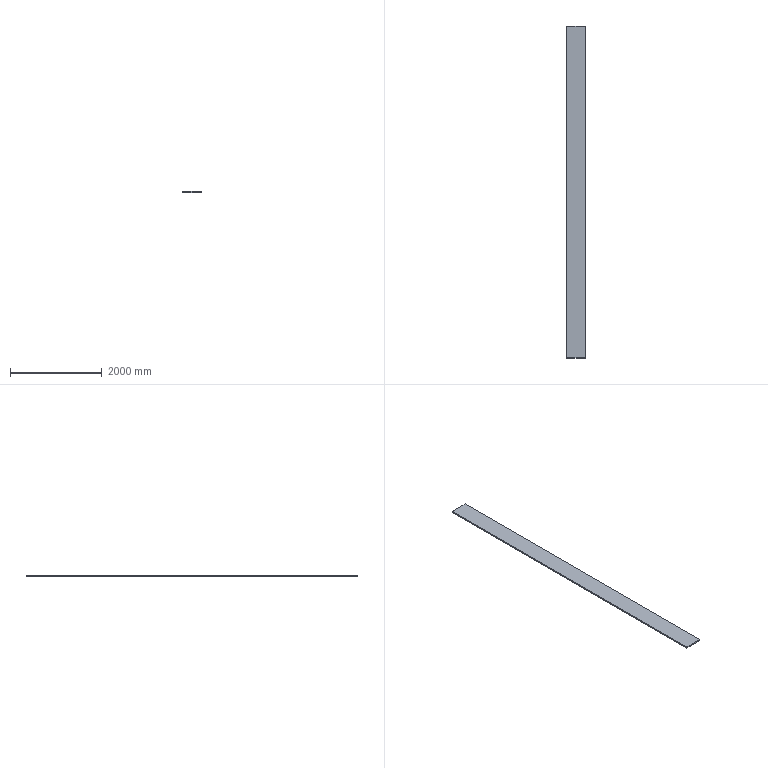Part | SolidWorks | features Extrusion 1 | 1 solid | 6 faces | box 400 x 7226 x 30 mm | volume 86712000 mm3 | plane 6
STEP:
#1=CARTESIAN_POINT('',(-200.,3613.,-15.));
#2=VERTEX_POINT('',#1);
#3=CARTESIAN_POINT('',(-200.,-3613.,-15.));
#4=VERTEX_POINT('',#3);
#5=CARTESIAN_POINT('',(-200.,3613.,-15.));
#6=DIRECTION('',(0.,-1.,0.));
#7=VECTOR('',#6,1000.);
#8=LINE('',#5,#7);
#9=EDGE_CURVE('',#2,#4,#8,.T.);
#10=ORIENTED_EDGE('',*,*,#9,.T.);
#11=CARTESIAN_POINT('',(-200.,-3613.,15.));
#12=VERTEX_POINT('',#11);
#13=CARTESIAN_POINT('',(-200.,-3613.,15.));
#14=DIRECTION('',(0.,0.,-1.));
#15=VECTOR('',#14,1000.);
#16=LINE('',#13,#15);
#17=EDGE_CURVE('',#12,#4,#16,.T.);
#18=ORIENTED_EDGE('',*,*,#17,.F.);
#19=CARTESIAN_POINT('',(-200.,3613.,15.));
#20=VERTEX_POINT('',#19);
#21=CARTESIAN_POINT('',(-200.,3613.,15.));
#22=DIRECTION('',(0.,-1.,0.));
#23=VECTOR('',#22,1000.);
#24=LINE('',#21,#23);
#25=EDGE_CURVE('',#20,#12,#24,.T.);
#26=ORIENTED_EDGE('',*,*,#25,.F.);
#27=CARTESIAN_POINT('',(-200.,3613.,15.));
#28=DIRECTION('',(0.,0.,-1.));
#29=VECTOR('',#28,1000.);
#30=LINE('',#27,#29);
#31=EDGE_CURVE('',#20,#2,#30,.T.);
#32=ORIENTED_EDGE('',*,*,#31,.T.);
#33=EDGE_LOOP('',(#10,#18,#26,#32));
#34=FACE_OUTER_BOUND('',#33,.T.);
#35=CARTESIAN_POINT('',(-200.,3613.,15.));
#36=DIRECTION('',(1.,0.,0.));
#37=DIRECTION('',(0.,1.,0.));
#38=AXIS2_PLACEMENT_3D('',#35,#36,#37);
#39=PLANE('',#38);
#40=ADVANCED_FACE('',(#34),#39,.F.);
#41=CARTESIAN_POINT('',(200.,-3613.,-15.));
#42=VERTEX_POINT('',#41);
#43=CARTESIAN_POINT('',(-200.,-3613.,-15.));
#44=DIRECTION('',(1.,0.,0.));
#45=VECTOR('',#44,1000.);
#46=LINE('',#43,#45);
#47=EDGE_CURVE('',#4,#42,#46,.T.);
#48=ORIENTED_EDGE('',*,*,#47,.T.);
#49=CARTESIAN_POINT('',(200.,-3613.,15.));
#50=VERTEX_POINT('',#49);
#51=CARTESIAN_POINT('',(200.,-3613.,15.));
#52=DIRECTION('',(0.,0.,-1.));
#53=VECTOR('',#52,1000.);
#54=LINE('',#51,#53);
#55=EDGE_CURVE('',#50,#42,#54,.T.);
#56=ORIENTED_EDGE('',*,*,#55,.F.);
#57=CARTESIAN_POINT('',(-200.,-3613.,15.));
#58=DIRECTION('',(1.,0.,0.));
#59=VECTOR('',#58,1000.);
#60=LINE('',#57,#59);
#61=EDGE_CURVE('',#12,#50,#60,.T.);
#62=ORIENTED_EDGE('',*,*,#61,.F.);
#63=ORIENTED_EDGE('',*,*,#17,.T.);
#64=EDGE_LOOP('',(#48,#56,#62,#63));
#65=FACE_OUTER_BOUND('',#64,.T.);
#66=CARTESIAN_POINT('',(-200.,-3613.,15.));
#67=DIRECTION('',(0.,1.,0.));
#68=DIRECTION('',(0.,0.,1.));
#69=AXIS2_PLACEMENT_3D('',#66,#67,#68);
#70=PLANE('',#69);
#71=ADVANCED_FACE('',(#65),#70,.F.);
#72=CARTESIAN_POINT('',(200.,3613.,-15.));
#73=VERTEX_POINT('',#72);
#74=CARTESIAN_POINT('',(200.,3613.,-15.));
#75=DIRECTION('',(0.,1.,0.));
#76=VECTOR('',#75,1000.);
#77=LINE('',#74,#76);
#78=EDGE_CURVE('',#42,#73,#77,.T.);
#79=ORIENTED_EDGE('',*,*,#78,.T.);
#80=CARTESIAN_POINT('',(200.,3613.,15.));
#81=VERTEX_POINT('',#80);
#82=CARTESIAN_POINT('',(200.,3613.,15.));
#83=DIRECTION('',(0.,0.,-1.));
#84=VECTOR('',#83,1000.);
#85=LINE('',#82,#84);
#86=EDGE_CURVE('',#81,#73,#85,.T.);
#87=ORIENTED_EDGE('',*,*,#86,.F.);
#88=CARTESIAN_POINT('',(200.,3613.,15.));
#89=DIRECTION('',(0.,1.,0.));
#90=VECTOR('',#89,1000.);
#91=LINE('',#88,#90);
#92=EDGE_CURVE('',#50,#81,#91,.T.);
#93=ORIENTED_EDGE('',*,*,#92,.F.);
#94=ORIENTED_EDGE('',*,*,#55,.T.);
#95=EDGE_LOOP('',(#79,#87,#93,#94));
#96=FACE_OUTER_BOUND('',#95,.T.);
#97=CARTESIAN_POINT('',(200.,3613.,15.));
#98=DIRECTION('',(-1.,0.,0.));
#99=DIRECTION('',(0.,-1.,0.));
#100=AXIS2_PLACEMENT_3D('',#97,#98,#99);
#101=PLANE('',#100);
#102=ADVANCED_FACE('',(#96),#101,.F.);
#103=CARTESIAN_POINT('',(-200.,3613.,-15.));
#104=DIRECTION('',(-1.,0.,0.));
#105=VECTOR('',#104,1000.);
#106=LINE('',#103,#105);
#107=EDGE_CURVE('',#73,#2,#106,.T.);
#108=ORIENTED_EDGE('',*,*,#107,.T.);
#109=ORIENTED_EDGE('',*,*,#31,.F.);
#110=CARTESIAN_POINT('',(-200.,3613.,15.));
#111=DIRECTION('',(-1.,0.,0.));
#112=VECTOR('',#111,1000.);
#113=LINE('',#110,#112);
#114=EDGE_CURVE('',#81,#20,#113,.T.);
#115=ORIENTED_EDGE('',*,*,#114,.F.);
#116=ORIENTED_EDGE('',*,*,#86,.T.);
#117=EDGE_LOOP('',(#108,#109,#115,#116));
#118=FACE_OUTER_BOUND('',#117,.T.);
#119=CARTESIAN_POINT('',(-200.,3613.,15.));
#120=DIRECTION('',(0.,-1.,0.));
#121=DIRECTION('',(0.,0.,-1.));
#122=AXIS2_PLACEMENT_3D('',#119,#120,#121);
#123=PLANE('',#122);
#124=ADVANCED_FACE('',(#118),#123,.F.);
#125=ORIENTED_EDGE('',*,*,#25,.T.);
#126=ORIENTED_EDGE('',*,*,#61,.T.);
#127=ORIENTED_EDGE('',*,*,#92,.T.);
#128=ORIENTED_EDGE('',*,*,#114,.T.);
#129=EDGE_LOOP('',(#125,#126,#127,#128));
#130=FACE_OUTER_BOUND('',#129,.T.);
#131=CARTESIAN_POINT('',(-200.,-3613.,15.));
#132=DIRECTION('',(0.,0.,1.));
#133=DIRECTION('',(1.,0.,0.));
#134=AXIS2_PLACEMENT_3D('',#131,#132,#133);
#135=PLANE('',#134);
#136=ADVANCED_FACE('',(#130),#135,.T.);
#137=ORIENTED_EDGE('',*,*,#9,.F.);
#138=ORIENTED_EDGE('',*,*,#107,.F.);
#139=ORIENTED_EDGE('',*,*,#78,.F.);
#140=ORIENTED_EDGE('',*,*,#47,.F.);
#141=EDGE_LOOP('',(#137,#138,#139,#140));
#142=FACE_OUTER_BOUND('',#141,.T.);
#143=CARTESIAN_POINT('',(-200.,-3613.,-15.));
#144=DIRECTION('',(0.,0.,1.));
#145=DIRECTION('',(1.,0.,0.));
#146=AXIS2_PLACEMENT_3D('',#143,#144,#145);
#147=PLANE('',#146);
#148=ADVANCED_FACE('',(#142),#147,.F.);
#149=CLOSED_SHELL('',(#40,#71,#102,#124,#136,#148));
#150=MANIFOLD_SOLID_BREP('',#149);
#151=CARTESIAN_POINT('',(0.,0.,0.));
#152=DIRECTION('',(0.,0.,1.));
#153=DIRECTION('',(1.,0.,0.));
#154=AXIS2_PLACEMENT_3D('',#151,#152,#153);
#155=(LENGTH_UNIT()NAMED_UNIT(*)SI_UNIT(.MILLI.,.METRE.));
#156=UNCERTAINTY_MEASURE_WITH_UNIT(LENGTH_MEASURE(0.00001),#155,'','');
#157=(NAMED_UNIT(*)PLANE_ANGLE_UNIT()SI_UNIT($,.RADIAN.));
#158=(NAMED_UNIT(*)SI_UNIT($,.STERADIAN.)SOLID_ANGLE_UNIT());
#159=(GEOMETRIC_REPRESENTATION_CONTEXT(3)GLOBAL_UNCERTAINTY_ASSIGNED_CONTEXT((#156))GLOBAL_UNIT_ASSIGNED_CONTEXT((#155,#157,#158))REPRESENTATION_CONTEXT('',''));
#160=ADVANCED_BREP_SHAPE_REPRESENTATION('',(#150,#154),#159);